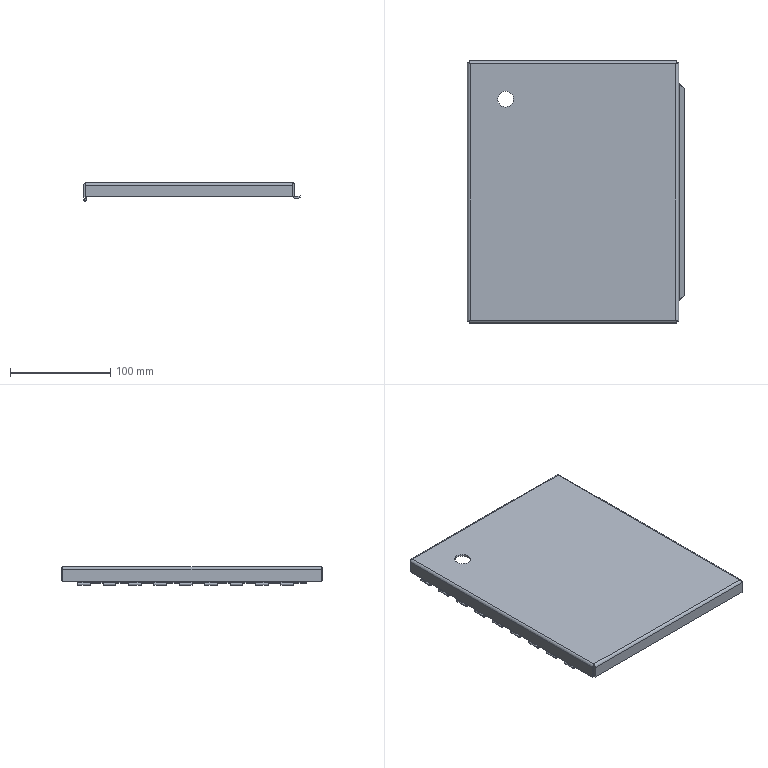Part | SolidWorks | features BaseBody 1 | 1 solid | 151 faces | box 216.967 x 261.925 x 18.699 mm | volume 126751 mm3 | plane 94 | cylinder 45 | spline 12 | commonest cylinder face diameters 1.27 x9 2.54 x9 2.921 x9 1.829 x7 5.486 x6 4.978 x3